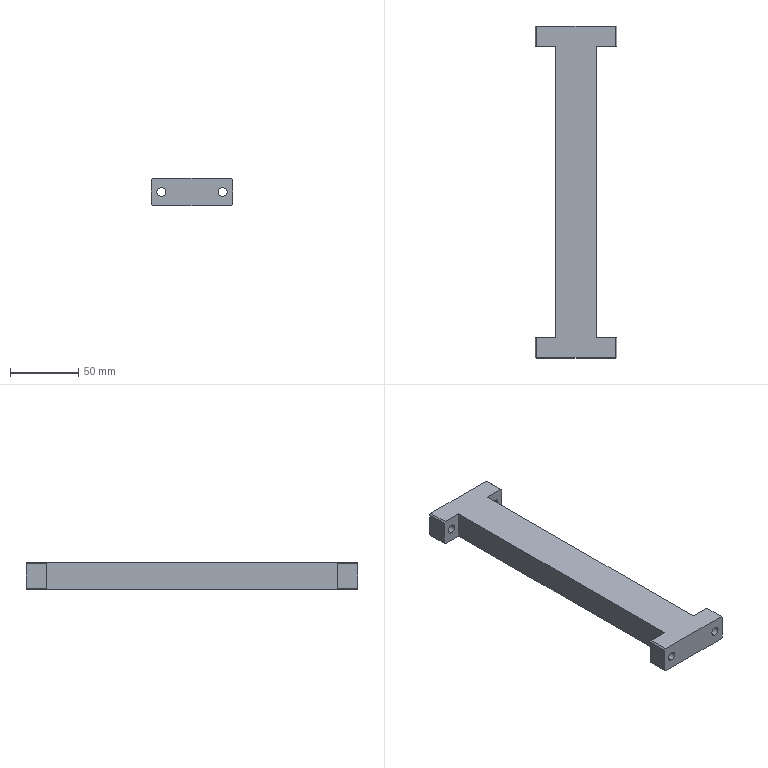Part | SolidWorks | features Chamfer 1, Extrusion 1, HoleWzd 1, ICE 1 | 1 solid | 30 faces | box 60 x 244 x 20 mm | volume 162287 mm3 | plane 22 | cylinder 8 | commonest cylinder face diameters 6.6 x8
STEP:
#1=CARTESIAN_POINT('',(-22.5,-122.,6.7));
#2=VERTEX_POINT('',#1);
#3=CARTESIAN_POINT('',(-22.5,-122.,13.3));
#4=VERTEX_POINT('',#3);
#5=CARTESIAN_POINT('',(-22.5,-122.,10.));
#6=DIRECTION('',(0.,1.,0.));
#7=DIRECTION('',(0.,0.,1.));
#8=AXIS2_PLACEMENT_3D('',#5,#6,#7);
#9=CIRCLE('',#8,3.3);
#10=EDGE_CURVE('',#2,#4,#9,.T.);
#11=ORIENTED_EDGE('',*,*,#10,.F.);
#12=CARTESIAN_POINT('',(-22.5,-107.,6.7));
#13=VERTEX_POINT('',#12);
#14=CARTESIAN_POINT('',(-22.5,122.,6.7));
#15=DIRECTION('',(0.,1.,0.));
#16=VECTOR('',#15,1000.);
#17=LINE('',#14,#16);
#18=EDGE_CURVE('',#2,#13,#17,.T.);
#19=ORIENTED_EDGE('',*,*,#18,.T.);
#20=CARTESIAN_POINT('',(-22.5,-107.,13.3));
#21=VERTEX_POINT('',#20);
#22=CARTESIAN_POINT('',(-22.5,-107.,10.));
#23=DIRECTION('',(0.,-1.,0.));
#24=DIRECTION('',(0.,0.,-1.));
#25=AXIS2_PLACEMENT_3D('',#22,#23,#24);
#26=CIRCLE('',#25,3.3);
#27=EDGE_CURVE('',#21,#13,#26,.T.);
#28=ORIENTED_EDGE('',*,*,#27,.F.);
#29=CARTESIAN_POINT('',(-22.5,122.,13.3));
#30=DIRECTION('',(0.,1.,0.));
#31=VECTOR('',#30,1000.);
#32=LINE('',#29,#31);
#33=EDGE_CURVE('',#4,#21,#32,.T.);
#34=ORIENTED_EDGE('',*,*,#33,.F.);
#35=EDGE_LOOP('',(#11,#19,#28,#34));
#36=FACE_OUTER_BOUND('',#35,.T.);
#37=CARTESIAN_POINT('',(-22.5,122.,10.));
#38=DIRECTION('',(0.,1.,0.));
#39=DIRECTION('',(0.,0.,1.));
#40=AXIS2_PLACEMENT_3D('',#37,#38,#39);
#41=CYLINDRICAL_SURFACE('',#40,3.3);
#42=ADVANCED_FACE('',(#36),#41,.F.);
#43=CARTESIAN_POINT('',(-22.5,107.,6.7));
#44=VERTEX_POINT('',#43);
#45=CARTESIAN_POINT('',(-22.5,107.,13.3));
#46=VERTEX_POINT('',#45);
#47=CARTESIAN_POINT('',(-22.5,107.,10.));
#48=DIRECTION('',(0.,1.,0.));
#49=DIRECTION('',(0.,0.,1.));
#50=AXIS2_PLACEMENT_3D('',#47,#48,#49);
#51=CIRCLE('',#50,3.3);
#52=EDGE_CURVE('',#44,#46,#51,.T.);
#53=ORIENTED_EDGE('',*,*,#52,.F.);
#54=CARTESIAN_POINT('',(-22.5,122.,6.7));
#55=VERTEX_POINT('',#54);
#56=CARTESIAN_POINT('',(-22.5,122.,6.7));
#57=DIRECTION('',(0.,1.,0.));
#58=VECTOR('',#57,1000.);
#59=LINE('',#56,#58);
#60=EDGE_CURVE('',#44,#55,#59,.T.);
#61=ORIENTED_EDGE('',*,*,#60,.T.);
#62=CARTESIAN_POINT('',(-22.5,122.,13.3));
#63=VERTEX_POINT('',#62);
#64=CARTESIAN_POINT('',(-22.5,122.,10.));
#65=DIRECTION('',(0.,1.,0.));
#66=DIRECTION('',(0.,0.,1.));
#67=AXIS2_PLACEMENT_3D('',#64,#65,#66);
#68=CIRCLE('',#67,3.3);
#69=EDGE_CURVE('',#55,#63,#68,.T.);
#70=ORIENTED_EDGE('',*,*,#69,.T.);
#71=CARTESIAN_POINT('',(-22.5,122.,13.3));
#72=DIRECTION('',(0.,1.,0.));
#73=VECTOR('',#72,1000.);
#74=LINE('',#71,#73);
#75=EDGE_CURVE('',#46,#63,#74,.T.);
#76=ORIENTED_EDGE('',*,*,#75,.F.);
#77=EDGE_LOOP('',(#53,#61,#70,#76));
#78=FACE_OUTER_BOUND('',#77,.T.);
#79=CARTESIAN_POINT('',(-22.5,122.,10.));
#80=DIRECTION('',(0.,1.,0.));
#81=DIRECTION('',(0.,0.,1.));
#82=AXIS2_PLACEMENT_3D('',#79,#80,#81);
#83=CYLINDRICAL_SURFACE('',#82,3.3);
#84=ADVANCED_FACE('',(#78),#83,.F.);
#85=CARTESIAN_POINT('',(22.5,107.,6.7));
#86=VERTEX_POINT('',#85);
#87=CARTESIAN_POINT('',(22.5,107.,13.3));
#88=VERTEX_POINT('',#87);
#89=CARTESIAN_POINT('',(22.5,107.,10.));
#90=DIRECTION('',(0.,1.,0.));
#91=DIRECTION('',(-1.,0.,0.));
#92=AXIS2_PLACEMENT_3D('',#89,#90,#91);
#93=CIRCLE('',#92,3.3);
#94=EDGE_CURVE('',#86,#88,#93,.T.);
#95=ORIENTED_EDGE('',*,*,#94,.F.);
#96=CARTESIAN_POINT('',(22.5,122.,6.7));
#97=VERTEX_POINT('',#96);
#98=CARTESIAN_POINT('',(22.5,122.,6.7));
#99=DIRECTION('',(0.,1.,0.));
#100=VECTOR('',#99,1000.);
#101=LINE('',#98,#100);
#102=EDGE_CURVE('',#86,#97,#101,.T.);
#103=ORIENTED_EDGE('',*,*,#102,.T.);
#104=CARTESIAN_POINT('',(22.5,122.,13.3));
#105=VERTEX_POINT('',#104);
#106=CARTESIAN_POINT('',(22.5,122.,10.));
#107=DIRECTION('',(0.,1.,0.));
#108=DIRECTION('',(0.,0.,1.));
#109=AXIS2_PLACEMENT_3D('',#106,#107,#108);
#110=CIRCLE('',#109,3.3);
#111=EDGE_CURVE('',#97,#105,#110,.T.);
#112=ORIENTED_EDGE('',*,*,#111,.T.);
#113=CARTESIAN_POINT('',(22.5,122.,13.3));
#114=DIRECTION('',(0.,1.,0.));
#115=VECTOR('',#114,1000.);
#116=LINE('',#113,#115);
#117=EDGE_CURVE('',#88,#105,#116,.T.);
#118=ORIENTED_EDGE('',*,*,#117,.F.);
#119=EDGE_LOOP('',(#95,#103,#112,#118));
#120=FACE_OUTER_BOUND('',#119,.T.);
#121=CARTESIAN_POINT('',(22.5,122.,10.));
#122=DIRECTION('',(0.,1.,0.));
#123=DIRECTION('',(0.,0.,1.));
#124=AXIS2_PLACEMENT_3D('',#121,#122,#123);
#125=CYLINDRICAL_SURFACE('',#124,3.3);
#126=ADVANCED_FACE('',(#120),#125,.F.);
#127=CARTESIAN_POINT('',(22.5,-122.,6.7));
#128=VERTEX_POINT('',#127);
#129=CARTESIAN_POINT('',(22.5,-122.,13.3));
#130=VERTEX_POINT('',#129);
#131=CARTESIAN_POINT('',(22.5,-122.,10.));
#132=DIRECTION('',(0.,1.,0.));
#133=DIRECTION('',(0.,0.,1.));
#134=AXIS2_PLACEMENT_3D('',#131,#132,#133);
#135=CIRCLE('',#134,3.3);
#136=EDGE_CURVE('',#128,#130,#135,.T.);
#137=ORIENTED_EDGE('',*,*,#136,.F.);
#138=CARTESIAN_POINT('',(22.5,-107.,6.7));
#139=VERTEX_POINT('',#138);
#140=CARTESIAN_POINT('',(22.5,122.,6.7));
#141=DIRECTION('',(0.,1.,0.));
#142=VECTOR('',#141,1000.);
#143=LINE('',#140,#142);
#144=EDGE_CURVE('',#128,#139,#143,.T.);
#145=ORIENTED_EDGE('',*,*,#144,.T.);
#146=CARTESIAN_POINT('',(22.5,-107.,13.3));
#147=VERTEX_POINT('',#146);
#148=CARTESIAN_POINT('',(22.5,-107.,10.));
#149=DIRECTION('',(0.,-1.,0.));
#150=DIRECTION('',(1.,0.,0.));
#151=AXIS2_PLACEMENT_3D('',#148,#149,#150);
#152=CIRCLE('',#151,3.3);
#153=EDGE_CURVE('',#147,#139,#152,.T.);
#154=ORIENTED_EDGE('',*,*,#153,.F.);
#155=CARTESIAN_POINT('',(22.5,122.,13.3));
#156=DIRECTION('',(0.,1.,0.));
#157=VECTOR('',#156,1000.);
#158=LINE('',#155,#157);
#159=EDGE_CURVE('',#130,#147,#158,.T.);
#160=ORIENTED_EDGE('',*,*,#159,.F.);
#161=EDGE_LOOP('',(#137,#145,#154,#160));
#162=FACE_OUTER_BOUND('',#161,.T.);
#163=CARTESIAN_POINT('',(22.5,122.,10.));
#164=DIRECTION('',(0.,1.,0.));
#165=DIRECTION('',(0.,0.,1.));
#166=AXIS2_PLACEMENT_3D('',#163,#164,#165);
#167=CYLINDRICAL_SURFACE('',#166,3.3);
#168=ADVANCED_FACE('',(#162),#167,.F.);
#169=CARTESIAN_POINT('',(30.,-122.,19.));
#170=VERTEX_POINT('',#169);
#171=CARTESIAN_POINT('',(30.,-122.,1.));
#172=VERTEX_POINT('',#171);
#173=CARTESIAN_POINT('',(30.,-122.,20.));
#174=DIRECTION('',(0.,0.,-1.));
#175=VECTOR('',#174,1000.);
#176=LINE('',#173,#175);
#177=EDGE_CURVE('',#170,#172,#176,.T.);
#178=ORIENTED_EDGE('',*,*,#177,.T.);
#179=CARTESIAN_POINT('',(30.,-107.,1.));
#180=VERTEX_POINT('',#179);
#181=CARTESIAN_POINT('',(30.,122.,1.));
#182=DIRECTION('',(0.,1.,0.));
#183=VECTOR('',#182,1000.);
#184=LINE('',#181,#183);
#185=EDGE_CURVE('',#172,#180,#184,.T.);
#186=ORIENTED_EDGE('',*,*,#185,.T.);
#187=CARTESIAN_POINT('',(30.,-107.,19.));
#188=VERTEX_POINT('',#187);
#189=CARTESIAN_POINT('',(30.,-107.,0.));
#190=DIRECTION('',(0.,0.,1.));
#191=VECTOR('',#190,1000.);
#192=LINE('',#189,#191);
#193=EDGE_CURVE('',#180,#188,#192,.T.);
#194=ORIENTED_EDGE('',*,*,#193,.T.);
#195=CARTESIAN_POINT('',(30.,-122.,19.));
#196=DIRECTION('',(0.,-1.,0.));
#197=VECTOR('',#196,1000.);
#198=LINE('',#195,#197);
#199=EDGE_CURVE('',#188,#170,#198,.T.);
#200=ORIENTED_EDGE('',*,*,#199,.T.);
#201=EDGE_LOOP('',(#178,#186,#194,#200));
#202=FACE_OUTER_BOUND('',#201,.T.);
#203=CARTESIAN_POINT('',(30.,122.,20.));
#204=DIRECTION('',(-1.,0.,0.));
#205=DIRECTION('',(0.,-1.,0.));
#206=AXIS2_PLACEMENT_3D('',#203,#204,#205);
#207=PLANE('',#206);
#208=ADVANCED_FACE('',(#202),#207,.F.);
#209=CARTESIAN_POINT('',(-30.,122.,19.));
#210=VERTEX_POINT('',#209);
#211=CARTESIAN_POINT('',(-30.,122.,1.));
#212=VERTEX_POINT('',#211);
#213=CARTESIAN_POINT('',(-30.,122.,20.));
#214=DIRECTION('',(0.,0.,-1.));
#215=VECTOR('',#214,1000.);
#216=LINE('',#213,#215);
#217=EDGE_CURVE('',#210,#212,#216,.T.);
#218=ORIENTED_EDGE('',*,*,#217,.T.);
#219=CARTESIAN_POINT('',(-30.,107.,1.));
#220=VERTEX_POINT('',#219);
#221=CARTESIAN_POINT('',(-30.,122.,1.));
#222=DIRECTION('',(0.,-1.,0.));
#223=VECTOR('',#222,1000.);
#224=LINE('',#221,#223);
#225=EDGE_CURVE('',#212,#220,#224,.T.);
#226=ORIENTED_EDGE('',*,*,#225,.T.);
#227=CARTESIAN_POINT('',(-30.,107.,19.));
#228=VERTEX_POINT('',#227);
#229=CARTESIAN_POINT('',(-30.,107.,0.));
#230=DIRECTION('',(0.,0.,1.));
#231=VECTOR('',#230,1000.);
#232=LINE('',#229,#231);
#233=EDGE_CURVE('',#220,#228,#232,.T.);
#234=ORIENTED_EDGE('',*,*,#233,.T.);
#235=CARTESIAN_POINT('',(-30.,122.,19.));
#236=DIRECTION('',(0.,1.,0.));
#237=VECTOR('',#236,1000.);
#238=LINE('',#235,#237);
#239=EDGE_CURVE('',#228,#210,#238,.T.);
#240=ORIENTED_EDGE('',*,*,#239,.T.);
#241=EDGE_LOOP('',(#218,#226,#234,#240));
#242=FACE_OUTER_BOUND('',#241,.T.);
#243=CARTESIAN_POINT('',(-30.,122.,20.));
#244=DIRECTION('',(1.,0.,0.));
#245=DIRECTION('',(0.,1.,0.));
#246=AXIS2_PLACEMENT_3D('',#243,#244,#245);
#247=PLANE('',#246);
#248=ADVANCED_FACE('',(#242),#247,.F.);
#249=CARTESIAN_POINT('',(30.,122.,19.));
#250=VERTEX_POINT('',#249);
#251=CARTESIAN_POINT('',(30.,122.,1.));
#252=VERTEX_POINT('',#251);
#253=CARTESIAN_POINT('',(30.,122.,20.));
#254=DIRECTION('',(0.,0.,-1.));
#255=VECTOR('',#254,1000.);
#256=LINE('',#253,#255);
#257=EDGE_CURVE('',#250,#252,#256,.T.);
#258=ORIENTED_EDGE('',*,*,#257,.F.);
#259=CARTESIAN_POINT('',(30.,107.,19.));
#260=VERTEX_POINT('',#259);
#261=CARTESIAN_POINT('',(30.,107.,19.));
#262=DIRECTION('',(0.,-1.,0.));
#263=VECTOR('',#262,1000.);
#264=LINE('',#261,#263);
#265=EDGE_CURVE('',#250,#260,#264,.T.);
#266=ORIENTED_EDGE('',*,*,#265,.T.);
#267=CARTESIAN_POINT('',(30.,107.,1.));
#268=VERTEX_POINT('',#267);
#269=CARTESIAN_POINT('',(30.,107.,0.));
#270=DIRECTION('',(0.,0.,1.));
#271=VECTOR('',#270,1000.);
#272=LINE('',#269,#271);
#273=EDGE_CURVE('',#268,#260,#272,.T.);
#274=ORIENTED_EDGE('',*,*,#273,.F.);
#275=CARTESIAN_POINT('',(30.,122.,1.));
#276=DIRECTION('',(0.,1.,0.));
#277=VECTOR('',#276,1000.);
#278=LINE('',#275,#277);
#279=EDGE_CURVE('',#268,#252,#278,.T.);
#280=ORIENTED_EDGE('',*,*,#279,.T.);
#281=EDGE_LOOP('',(#258,#266,#274,#280));
#282=FACE_OUTER_BOUND('',#281,.T.);
#283=CARTESIAN_POINT('',(30.,122.,20.));
#284=DIRECTION('',(-1.,0.,0.));
#285=DIRECTION('',(0.,-1.,0.));
#286=AXIS2_PLACEMENT_3D('',#283,#284,#285);
#287=PLANE('',#286);
#288=ADVANCED_FACE('',(#282),#287,.F.);
#289=CARTESIAN_POINT('',(-22.5,122.,10.));
#290=DIRECTION('',(0.,1.,0.));
#291=DIRECTION('',(0.,0.,1.));
#292=AXIS2_PLACEMENT_3D('',#289,#290,#291);
#293=CIRCLE('',#292,3.3);
#294=EDGE_CURVE('',#63,#55,#293,.T.);
#295=ORIENTED_EDGE('',*,*,#294,.F.);
#296=ORIENTED_EDGE('',*,*,#69,.F.);
#297=EDGE_LOOP('',(#295,#296));
#298=FACE_BOUND('',#297,.T.);
#299=CARTESIAN_POINT('',(22.5,122.,10.));
#300=DIRECTION('',(0.,1.,0.));
#301=DIRECTION('',(0.,0.,1.));
#302=AXIS2_PLACEMENT_3D('',#299,#300,#301);
#303=CIRCLE('',#302,3.3);
#304=EDGE_CURVE('',#105,#97,#303,.T.);
#305=ORIENTED_EDGE('',*,*,#304,.F.);
#306=ORIENTED_EDGE('',*,*,#111,.F.);
#307=EDGE_LOOP('',(#305,#306));
#308=FACE_BOUND('',#307,.T.);
#309=CARTESIAN_POINT('',(29.,122.,20.));
#310=VERTEX_POINT('',#309);
#311=CARTESIAN_POINT('',(-29.,122.,20.));
#312=VERTEX_POINT('',#311);
#313=CARTESIAN_POINT('',(-30.,122.,20.));
#314=DIRECTION('',(-1.,0.,0.));
#315=VECTOR('',#314,1000.);
#316=LINE('',#313,#315);
#317=EDGE_CURVE('',#310,#312,#316,.T.);
#318=ORIENTED_EDGE('',*,*,#317,.F.);
#319=CARTESIAN_POINT('',(29.,122.,20.));
#320=DIRECTION('',(0.7071,0.,-0.7071));
#321=VECTOR('',#320,1000.);
#322=LINE('',#319,#321);
#323=EDGE_CURVE('',#310,#250,#322,.T.);
#324=ORIENTED_EDGE('',*,*,#323,.T.);
#325=ORIENTED_EDGE('',*,*,#257,.T.);
#326=CARTESIAN_POINT('',(29.,122.,0.));
#327=VERTEX_POINT('',#326);
#328=CARTESIAN_POINT('',(30.,122.,1.));
#329=DIRECTION('',(-0.7071,0.,-0.7071));
#330=VECTOR('',#329,1000.);
#331=LINE('',#328,#330);
#332=EDGE_CURVE('',#252,#327,#331,.T.);
#333=ORIENTED_EDGE('',*,*,#332,.T.);
#334=CARTESIAN_POINT('',(-29.,122.,0.));
#335=VERTEX_POINT('',#334);
#336=CARTESIAN_POINT('',(-30.,122.,0.));
#337=DIRECTION('',(-1.,0.,0.));
#338=VECTOR('',#337,1000.);
#339=LINE('',#336,#338);
#340=EDGE_CURVE('',#327,#335,#339,.T.);
#341=ORIENTED_EDGE('',*,*,#340,.T.);
#342=CARTESIAN_POINT('',(-30.,122.,1.));
#343=DIRECTION('',(-0.7071,0.,0.7071));
#344=VECTOR('',#343,1000.);
#345=LINE('',#342,#344);
#346=EDGE_CURVE('',#335,#212,#345,.T.);
#347=ORIENTED_EDGE('',*,*,#346,.T.);
#348=ORIENTED_EDGE('',*,*,#217,.F.);
#349=CARTESIAN_POINT('',(-29.,122.,20.));
#350=DIRECTION('',(0.7071,0.,0.7071));
#351=VECTOR('',#350,1000.);
#352=LINE('',#349,#351);
#353=EDGE_CURVE('',#210,#312,#352,.T.);
#354=ORIENTED_EDGE('',*,*,#353,.T.);
#355=EDGE_LOOP('',(#318,#324,#325,#333,#341,#347,#348,#354));
#356=FACE_OUTER_BOUND('',#355,.T.);
#357=CARTESIAN_POINT('',(-30.,122.,20.));
#358=DIRECTION('',(0.,-1.,0.));
#359=DIRECTION('',(0.,0.,-1.));
#360=AXIS2_PLACEMENT_3D('',#357,#358,#359);
#361=PLANE('',#360);
#362=ADVANCED_FACE('',(#298,#308,#356),#361,.F.);
#363=CARTESIAN_POINT('',(-30.,-122.,19.));
#364=VERTEX_POINT('',#363);
#365=CARTESIAN_POINT('',(-30.,-122.,1.));
#366=VERTEX_POINT('',#365);
#367=CARTESIAN_POINT('',(-30.,-122.,20.));
#368=DIRECTION('',(0.,0.,-1.));
#369=VECTOR('',#368,1000.);
#370=LINE('',#367,#369);
#371=EDGE_CURVE('',#364,#366,#370,.T.);
#372=ORIENTED_EDGE('',*,*,#371,.F.);
#373=CARTESIAN_POINT('',(-30.,-107.,19.));
#374=VERTEX_POINT('',#373);
#375=CARTESIAN_POINT('',(-30.,-107.,19.));
#376=DIRECTION('',(0.,1.,0.));
#377=VECTOR('',#376,1000.);
#378=LINE('',#375,#377);
#379=EDGE_CURVE('',#364,#374,#378,.T.);
#380=ORIENTED_EDGE('',*,*,#379,.T.);
#381=CARTESIAN_POINT('',(-30.,-107.,1.));
#382=VERTEX_POINT('',#381);
#383=CARTESIAN_POINT('',(-30.,-107.,0.));
#384=DIRECTION('',(0.,0.,1.));
#385=VECTOR('',#384,1000.);
#386=LINE('',#383,#385);
#387=EDGE_CURVE('',#382,#374,#386,.T.);
#388=ORIENTED_EDGE('',*,*,#387,.F.);
#389=CARTESIAN_POINT('',(-30.,122.,1.));
#390=DIRECTION('',(0.,-1.,0.));
#391=VECTOR('',#390,1000.);
#392=LINE('',#389,#391);
#393=EDGE_CURVE('',#382,#366,#392,.T.);
#394=ORIENTED_EDGE('',*,*,#393,.T.);
#395=EDGE_LOOP('',(#372,#380,#388,#394));
#396=FACE_OUTER_BOUND('',#395,.T.);
#397=CARTESIAN_POINT('',(-30.,122.,20.));
#398=DIRECTION('',(1.,0.,0.));
#399=DIRECTION('',(0.,1.,0.));
#400=AXIS2_PLACEMENT_3D('',#397,#398,#399);
#401=PLANE('',#400);
#402=ADVANCED_FACE('',(#396),#401,.F.);
#403=CARTESIAN_POINT('',(-22.5,-122.,10.));
#404=DIRECTION('',(0.,1.,0.));
#405=DIRECTION('',(0.,0.,1.));
#406=AXIS2_PLACEMENT_3D('',#403,#404,#405);
#407=CIRCLE('',#406,3.3);
#408=EDGE_CURVE('',#4,#2,#407,.T.);
#409=ORIENTED_EDGE('',*,*,#408,.T.);
#410=ORIENTED_EDGE('',*,*,#10,.T.);
#411=EDGE_LOOP('',(#409,#410));
#412=FACE_BOUND('',#411,.T.);
#413=CARTESIAN_POINT('',(22.5,-122.,10.));
#414=DIRECTION('',(0.,1.,0.));
#415=DIRECTION('',(0.,0.,1.));
#416=AXIS2_PLACEMENT_3D('',#413,#414,#415);
#417=CIRCLE('',#416,3.3);
#418=EDGE_CURVE('',#130,#128,#417,.T.);
#419=ORIENTED_EDGE('',*,*,#418,.T.);
#420=ORIENTED_EDGE('',*,*,#136,.T.);
#421=EDGE_LOOP('',(#419,#420));
#422=FACE_BOUND('',#421,.T.);
#423=CARTESIAN_POINT('',(-29.,-122.,20.));
#424=VERTEX_POINT('',#423);
#425=CARTESIAN_POINT('',(29.,-122.,20.));
#426=VERTEX_POINT('',#425);
#427=CARTESIAN_POINT('',(-30.,-122.,20.));
#428=DIRECTION('',(1.,0.,0.));
#429=VECTOR('',#428,1000.);
#430=LINE('',#427,#429);
#431=EDGE_CURVE('',#424,#426,#430,.T.);
#432=ORIENTED_EDGE('',*,*,#431,.F.);
#433=CARTESIAN_POINT('',(-29.,-122.,20.));
#434=DIRECTION('',(-0.7071,0.,-0.7071));
#435=VECTOR('',#434,1000.);
#436=LINE('',#433,#435);
#437=EDGE_CURVE('',#424,#364,#436,.T.);
#438=ORIENTED_EDGE('',*,*,#437,.T.);
#439=ORIENTED_EDGE('',*,*,#371,.T.);
#440=CARTESIAN_POINT('',(-29.,-122.,0.));
#441=VERTEX_POINT('',#440);
#442=CARTESIAN_POINT('',(-30.,-122.,1.));
#443=DIRECTION('',(0.7071,0.,-0.7071));
#444=VECTOR('',#443,1000.);
#445=LINE('',#442,#444);
#446=EDGE_CURVE('',#366,#441,#445,.T.);
#447=ORIENTED_EDGE('',*,*,#446,.T.);
#448=CARTESIAN_POINT('',(29.,-122.,0.));
#449=VERTEX_POINT('',#448);
#450=CARTESIAN_POINT('',(-30.,-122.,0.));
#451=DIRECTION('',(1.,0.,0.));
#452=VECTOR('',#451,1000.);
#453=LINE('',#450,#452);
#454=EDGE_CURVE('',#441,#449,#453,.T.);
#455=ORIENTED_EDGE('',*,*,#454,.T.);
#456=CARTESIAN_POINT('',(30.,-122.,1.));
#457=DIRECTION('',(0.7071,0.,0.7071));
#458=VECTOR('',#457,1000.);
#459=LINE('',#456,#458);
#460=EDGE_CURVE('',#449,#172,#459,.T.);
#461=ORIENTED_EDGE('',*,*,#460,.T.);
#462=ORIENTED_EDGE('',*,*,#177,.F.);
#463=CARTESIAN_POINT('',(29.,-122.,20.));
#464=DIRECTION('',(-0.7071,0.,0.7071));
#465=VECTOR('',#464,1000.);
#466=LINE('',#463,#465);
#467=EDGE_CURVE('',#170,#426,#466,.T.);
#468=ORIENTED_EDGE('',*,*,#467,.T.);
#469=EDGE_LOOP('',(#432,#438,#439,#447,#455,#461,#462,#468));
#470=FACE_OUTER_BOUND('',#469,.T.);
#471=CARTESIAN_POINT('',(-30.,-122.,20.));
#472=DIRECTION('',(0.,1.,0.));
#473=DIRECTION('',(0.,0.,1.));
#474=AXIS2_PLACEMENT_3D('',#471,#472,#473);
#475=PLANE('',#474);
#476=ADVANCED_FACE('',(#412,#422,#470),#475,.F.);
#477=CARTESIAN_POINT('',(-29.,-107.,20.));
#478=VERTEX_POINT('',#477);
#479=CARTESIAN_POINT('',(-15.,-107.,20.));
#480=VERTEX_POINT('',#479);
#481=CARTESIAN_POINT('',(-30.,-107.,20.));
#482=DIRECTION('',(1.,0.,0.));
#483=VECTOR('',#482,1000.);
#484=LINE('',#481,#483);
#485=EDGE_CURVE('',#478,#480,#484,.T.);
#486=ORIENTED_EDGE('',*,*,#485,.F.);
#487=CARTESIAN_POINT('',(-29.,-122.,20.));
#488=DIRECTION('',(0.,-1.,0.));
#489=VECTOR('',#488,1000.);
#490=LINE('',#487,#489);
#491=EDGE_CURVE('',#478,#424,#490,.T.);
#492=ORIENTED_EDGE('',*,*,#491,.T.);
#493=ORIENTED_EDGE('',*,*,#431,.T.);
#494=CARTESIAN_POINT('',(29.,-107.,20.));
#495=VERTEX_POINT('',#494);
#496=CARTESIAN_POINT('',(29.,-107.,20.));
#497=DIRECTION('',(0.,1.,0.));
#498=VECTOR('',#497,1000.);
#499=LINE('',#496,#498);
#500=EDGE_CURVE('',#426,#495,#499,.T.);
#501=ORIENTED_EDGE('',*,*,#500,.T.);
#502=CARTESIAN_POINT('',(15.,-107.,20.));
#503=VERTEX_POINT('',#502);
#504=CARTESIAN_POINT('',(30.,-107.,20.));
#505=DIRECTION('',(1.,0.,0.));
#506=VECTOR('',#505,1000.);
#507=LINE('',#504,#506);
#508=EDGE_CURVE('',#503,#495,#507,.T.);
#509=ORIENTED_EDGE('',*,*,#508,.F.);
#510=CARTESIAN_POINT('',(15.,107.,20.));
#511=VERTEX_POINT('',#510);
#512=CARTESIAN_POINT('',(15.,107.,20.));
#513=DIRECTION('',(0.,-1.,0.));
#514=VECTOR('',#513,1000.);
#515=LINE('',#512,#514);
#516=EDGE_CURVE('',#511,#503,#515,.T.);
#517=ORIENTED_EDGE('',*,*,#516,.F.);
#518=CARTESIAN_POINT('',(29.,107.,20.));
#519=VERTEX_POINT('',#518);
#520=CARTESIAN_POINT('',(30.,107.,20.));
#521=DIRECTION('',(-1.,0.,0.));
#522=VECTOR('',#521,1000.);
#523=LINE('',#520,#522);
#524=EDGE_CURVE('',#519,#511,#523,.T.);
#525=ORIENTED_EDGE('',*,*,#524,.F.);
#526=CARTESIAN_POINT('',(29.,122.,20.));
#527=DIRECTION('',(0.,1.,0.));
#528=VECTOR('',#527,1000.);
#529=LINE('',#526,#528);
#530=EDGE_CURVE('',#519,#310,#529,.T.);
#531=ORIENTED_EDGE('',*,*,#530,.T.);
#532=ORIENTED_EDGE('',*,*,#317,.T.);
#533=CARTESIAN_POINT('',(-29.,107.,20.));
#534=VERTEX_POINT('',#533);
#535=CARTESIAN_POINT('',(-29.,107.,20.));
#536=DIRECTION('',(0.,-1.,0.));
#537=VECTOR('',#536,1000.);
#538=LINE('',#535,#537);
#539=EDGE_CURVE('',#312,#534,#538,.T.);
#540=ORIENTED_EDGE('',*,*,#539,.T.);
#541=CARTESIAN_POINT('',(-15.,107.,20.));
#542=VERTEX_POINT('',#541);
#543=CARTESIAN_POINT('',(-30.,107.,20.));
#544=DIRECTION('',(-1.,0.,0.));
#545=VECTOR('',#544,1000.);
#546=LINE('',#543,#545);
#547=EDGE_CURVE('',#542,#534,#546,.T.);
#548=ORIENTED_EDGE('',*,*,#547,.F.);
#549=CARTESIAN_POINT('',(-15.,107.,20.));
#550=DIRECTION('',(0.,1.,0.));
#551=VECTOR('',#550,1000.);
#552=LINE('',#549,#551);
#553=EDGE_CURVE('',#480,#542,#552,.T.);
#554=ORIENTED_EDGE('',*,*,#553,.F.);
#555=EDGE_LOOP('',(#486,#492,#493,#501,#509,#517,#525,#531,#532,#540,#548,#554));
#556=FACE_OUTER_BOUND('',#555,.T.);
#557=CARTESIAN_POINT('',(0.,0.,20.));
#558=DIRECTION('',(0.,0.,1.));
#559=DIRECTION('',(1.,0.,0.));
#560=AXIS2_PLACEMENT_3D('',#557,#558,#559);
#561=PLANE('',#560);
#562=ADVANCED_FACE('',(#556),#561,.T.);
#563=ORIENTED_EDGE('',*,*,#454,.F.);
#564=CARTESIAN_POINT('',(-29.,-107.,0.));
#565=VERTEX_POINT('',#564);
#566=CARTESIAN_POINT('',(-29.,0.,0.));
#567=DIRECTION('',(0.,1.,0.));
#568=VECTOR('',#567,1000.);
#569=LINE('',#566,#568);
#570=EDGE_CURVE('',#441,#565,#569,.T.);
#571=ORIENTED_EDGE('',*,*,#570,.T.);
#572=CARTESIAN_POINT('',(-15.,-107.,0.));
#573=VERTEX_POINT('',#572);
#574=CARTESIAN_POINT('',(-30.,-107.,0.));
#575=DIRECTION('',(1.,0.,0.));
#576=VECTOR('',#575,1000.);
#577=LINE('',#574,#576);
#578=EDGE_CURVE('',#565,#573,#577,.T.);
#579=ORIENTED_EDGE('',*,*,#578,.T.);
#580=CARTESIAN_POINT('',(-15.,107.,0.));
#581=VERTEX_POINT('',#580);
#582=CARTESIAN_POINT('',(-15.,107.,0.));
#583=DIRECTION('',(0.,1.,0.));
#584=VECTOR('',#583,1000.);
#585=LINE('',#582,#584);
#586=EDGE_CURVE('',#573,#581,#585,.T.);
#587=ORIENTED_EDGE('',*,*,#586,.T.);
#588=CARTESIAN_POINT('',(-29.,107.,0.));
#589=VERTEX_POINT('',#588);
#590=CARTESIAN_POINT('',(-30.,107.,0.));
#591=DIRECTION('',(-1.,0.,0.));
#592=VECTOR('',#591,1000.);
#593=LINE('',#590,#592);
#594=EDGE_CURVE('',#581,#589,#593,.T.);
#595=ORIENTED_EDGE('',*,*,#594,.T.);
#596=CARTESIAN_POINT('',(-29.,0.,0.));
#597=DIRECTION('',(0.,1.,0.));
#598=VECTOR('',#597,1000.);
#599=LINE('',#596,#598);
#600=EDGE_CURVE('',#589,#335,#599,.T.);
#601=ORIENTED_EDGE('',*,*,#600,.T.);
#602=ORIENTED_EDGE('',*,*,#340,.F.);
#603=CARTESIAN_POINT('',(29.,107.,0.));
#604=VERTEX_POINT('',#603);
#605=CARTESIAN_POINT('',(29.,0.,0.));
#606=DIRECTION('',(0.,-1.,0.));
#607=VECTOR('',#606,1000.);
#608=LINE('',#605,#607);
#609=EDGE_CURVE('',#327,#604,#608,.T.);
#610=ORIENTED_EDGE('',*,*,#609,.T.);
#611=CARTESIAN_POINT('',(15.,107.,0.));
#612=VERTEX_POINT('',#611);
#613=CARTESIAN_POINT('',(30.,107.,0.));
#614=DIRECTION('',(-1.,0.,0.));
#615=VECTOR('',#614,1000.);
#616=LINE('',#613,#615);
#617=EDGE_CURVE('',#604,#612,#616,.T.);
#618=ORIENTED_EDGE('',*,*,#617,.T.);
#619=CARTESIAN_POINT('',(15.,-107.,0.));
#620=VERTEX_POINT('',#619);
#621=CARTESIAN_POINT('',(15.,107.,0.));
#622=DIRECTION('',(0.,-1.,0.));
#623=VECTOR('',#622,1000.);
#624=LINE('',#621,#623);
#625=EDGE_CURVE('',#612,#620,#624,.T.);
#626=ORIENTED_EDGE('',*,*,#625,.T.);
#627=CARTESIAN_POINT('',(29.,-107.,0.));
#628=VERTEX_POINT('',#627);
#629=CARTESIAN_POINT('',(30.,-107.,0.));
#630=DIRECTION('',(1.,0.,0.));
#631=VECTOR('',#630,1000.);
#632=LINE('',#629,#631);
#633=EDGE_CURVE('',#620,#628,#632,.T.);
#634=ORIENTED_EDGE('',*,*,#633,.T.);
#635=CARTESIAN_POINT('',(29.,0.,0.));
#636=DIRECTION('',(0.,-1.,0.));
#637=VECTOR('',#636,1000.);
#638=LINE('',#635,#637);
#639=EDGE_CURVE('',#628,#449,#638,.T.);
#640=ORIENTED_EDGE('',*,*,#639,.T.);
#641=EDGE_LOOP('',(#563,#571,#579,#587,#595,#601,#602,#610,#618,#626,#634,#640));
#642=FACE_OUTER_BOUND('',#641,.T.);
#643=CARTESIAN_POINT('',(0.,0.,0.));
#644=DIRECTION('',(0.,0.,1.));
#645=DIRECTION('',(1.,0.,0.));
#646=AXIS2_PLACEMENT_3D('',#643,#644,#645);
#647=PLANE('',#646);
#648=ADVANCED_FACE('',(#642),#647,.F.);
#649=ORIENTED_EDGE('',*,*,#153,.T.);
#650=CARTESIAN_POINT('',(22.5,-107.,10.));
#651=DIRECTION('',(0.,-1.,0.));
#652=DIRECTION('',(1.,0.,0.));
#653=AXIS2_PLACEMENT_3D('',#650,#651,#652);
#654=CIRCLE('',#653,3.3);
#655=EDGE_CURVE('',#139,#147,#654,.T.);
#656=ORIENTED_EDGE('',*,*,#655,.T.);
#657=EDGE_LOOP('',(#649,#656));
#658=FACE_BOUND('',#657,.T.);
#659=ORIENTED_EDGE('',*,*,#193,.F.);
#660=CARTESIAN_POINT('',(30.,-107.,1.));
#661=DIRECTION('',(-0.7071,0.,-0.7071));
#662=VECTOR('',#661,1000.);
#663=LINE('',#660,#662);
#664=EDGE_CURVE('',#180,#628,#663,.T.);
#665=ORIENTED_EDGE('',*,*,#664,.T.);
#666=ORIENTED_EDGE('',*,*,#633,.F.);
#667=CARTESIAN_POINT('',(15.,-107.,0.));
#668=DIRECTION('',(0.,0.,1.));
#669=VECTOR('',#668,1000.);
#670=LINE('',#667,#669);
#671=EDGE_CURVE('',#620,#503,#670,.T.);
#672=ORIENTED_EDGE('',*,*,#671,.T.);
#673=ORIENTED_EDGE('',*,*,#508,.T.);
#674=CARTESIAN_POINT('',(29.,-107.,20.));
#675=DIRECTION('',(0.7071,0.,-0.7071));
#676=VECTOR('',#675,1000.);
#677=LINE('',#674,#676);
#678=EDGE_CURVE('',#495,#188,#677,.T.);
#679=ORIENTED_EDGE('',*,*,#678,.T.);
#680=EDGE_LOOP('',(#659,#665,#666,#672,#673,#679));
#681=FACE_OUTER_BOUND('',#680,.T.);
#682=CARTESIAN_POINT('',(30.,-107.,0.));
#683=DIRECTION('',(0.,-1.,0.));
#684=DIRECTION('',(1.,0.,0.));
#685=AXIS2_PLACEMENT_3D('',#682,#683,#684);
#686=PLANE('',#685);
#687=ADVANCED_FACE('',(#658,#681),#686,.F.);
#688=ORIENTED_EDGE('',*,*,#516,.T.);
#689=ORIENTED_EDGE('',*,*,#671,.F.);
#690=ORIENTED_EDGE('',*,*,#625,.F.);
#691=CARTESIAN_POINT('',(15.,107.,0.));
#692=DIRECTION('',(0.,0.,1.));
#693=VECTOR('',#692,1000.);
#694=LINE('',#691,#693);
#695=EDGE_CURVE('',#612,#511,#694,.T.);
#696=ORIENTED_EDGE('',*,*,#695,.T.);
#697=EDGE_LOOP('',(#688,#689,#690,#696));
#698=FACE_OUTER_BOUND('',#697,.T.);
#699=CARTESIAN_POINT('',(15.,107.,0.));
#700=DIRECTION('',(-1.,0.,0.));
#701=DIRECTION('',(0.,0.,1.));
#702=AXIS2_PLACEMENT_3D('',#699,#700,#701);
#703=PLANE('',#702);
#704=ADVANCED_FACE('',(#698),#703,.F.);
#705=CARTESIAN_POINT('',(22.5,107.,10.));
#706=DIRECTION('',(0.,1.,0.));
#707=DIRECTION('',(-1.,0.,0.));
#708=AXIS2_PLACEMENT_3D('',#705,#706,#707);
#709=CIRCLE('',#708,3.3);
#710=EDGE_CURVE('',#88,#86,#709,.T.);
#711=ORIENTED_EDGE('',*,*,#710,.T.);
#712=ORIENTED_EDGE('',*,*,#94,.T.);
#713=EDGE_LOOP('',(#711,#712));
#714=FACE_BOUND('',#713,.T.);
#715=ORIENTED_EDGE('',*,*,#273,.T.);
#716=CARTESIAN_POINT('',(29.,107.,20.));
#717=DIRECTION('',(-0.7071,0.,0.7071));
#718=VECTOR('',#717,1000.);
#719=LINE('',#716,#718);
#720=EDGE_CURVE('',#260,#519,#719,.T.);
#721=ORIENTED_EDGE('',*,*,#720,.T.);
#722=ORIENTED_EDGE('',*,*,#524,.T.);
#723=ORIENTED_EDGE('',*,*,#695,.F.);
#724=ORIENTED_EDGE('',*,*,#617,.F.);
#725=CARTESIAN_POINT('',(30.,107.,1.));
#726=DIRECTION('',(0.7071,0.,0.7071));
#727=VECTOR('',#726,1000.);
#728=LINE('',#725,#727);
#729=EDGE_CURVE('',#604,#268,#728,.T.);
#730=ORIENTED_EDGE('',*,*,#729,.T.);
#731=EDGE_LOOP('',(#715,#721,#722,#723,#724,#730));
#732=FACE_OUTER_BOUND('',#731,.T.);
#733=CARTESIAN_POINT('',(30.,107.,0.));
#734=DIRECTION('',(0.,1.,0.));
#735=DIRECTION('',(-1.,0.,0.));
#736=AXIS2_PLACEMENT_3D('',#733,#734,#735);
#737=PLANE('',#736);
#738=ADVANCED_FACE('',(#714,#732),#737,.F.);
#739=CARTESIAN_POINT('',(-22.5,107.,10.));
#740=DIRECTION('',(0.,1.,0.));
#741=DIRECTION('',(0.,0.,1.));
#742=AXIS2_PLACEMENT_3D('',#739,#740,#741);
#743=CIRCLE('',#742,3.3);
#744=EDGE_CURVE('',#46,#44,#743,.T.);
#745=ORIENTED_EDGE('',*,*,#744,.T.);
#746=ORIENTED_EDGE('',*,*,#52,.T.);
#747=EDGE_LOOP('',(#745,#746));
#748=FACE_BOUND('',#747,.T.);
#749=ORIENTED_EDGE('',*,*,#233,.F.);
#750=CARTESIAN_POINT('',(-30.,107.,1.));
#751=DIRECTION('',(0.7071,0.,-0.7071));
#752=VECTOR('',#751,1000.);
#753=LINE('',#750,#752);
#754=EDGE_CURVE('',#220,#589,#753,.T.);
#755=ORIENTED_EDGE('',*,*,#754,.T.);
#756=ORIENTED_EDGE('',*,*,#594,.F.);
#757=CARTESIAN_POINT('',(-15.,107.,0.));
#758=DIRECTION('',(0.,0.,1.));
#759=VECTOR('',#758,1000.);
#760=LINE('',#757,#759);
#761=EDGE_CURVE('',#581,#542,#760,.T.);
#762=ORIENTED_EDGE('',*,*,#761,.T.);
#763=ORIENTED_EDGE('',*,*,#547,.T.);
#764=CARTESIAN_POINT('',(-29.,107.,20.));
#765=DIRECTION('',(-0.7071,0.,-0.7071));
#766=VECTOR('',#765,1000.);
#767=LINE('',#764,#766);
#768=EDGE_CURVE('',#534,#228,#767,.T.);
#769=ORIENTED_EDGE('',*,*,#768,.T.);
#770=EDGE_LOOP('',(#749,#755,#756,#762,#763,#769));
#771=FACE_OUTER_BOUND('',#770,.T.);
#772=CARTESIAN_POINT('',(-30.,107.,0.));
#773=DIRECTION('',(0.,1.,0.));
#774=DIRECTION('',(0.,0.,1.));
#775=AXIS2_PLACEMENT_3D('',#772,#773,#774);
#776=PLANE('',#775);
#777=ADVANCED_FACE('',(#748,#771),#776,.F.);
#778=ORIENTED_EDGE('',*,*,#553,.T.);
#779=ORIENTED_EDGE('',*,*,#761,.F.);
#780=ORIENTED_EDGE('',*,*,#586,.F.);
#781=CARTESIAN_POINT('',(-15.,-107.,0.));
#782=DIRECTION('',(0.,0.,1.));
#783=VECTOR('',#782,1000.);
#784=LINE('',#781,#783);
#785=EDGE_CURVE('',#573,#480,#784,.T.);
#786=ORIENTED_EDGE('',*,*,#785,.T.);
#787=EDGE_LOOP('',(#778,#779,#780,#786));
#788=FACE_OUTER_BOUND('',#787,.T.);
#789=CARTESIAN_POINT('',(-15.,107.,0.));
#790=DIRECTION('',(1.,0.,0.));
#791=DIRECTION('',(0.,0.,-1.));
#792=AXIS2_PLACEMENT_3D('',#789,#790,#791);
#793=PLANE('',#792);
#794=ADVANCED_FACE('',(#788),#793,.F.);
#795=ORIENTED_EDGE('',*,*,#27,.T.);
#796=CARTESIAN_POINT('',(-22.5,-107.,10.));
#797=DIRECTION('',(0.,-1.,0.));
#798=DIRECTION('',(0.,0.,-1.));
#799=AXIS2_PLACEMENT_3D('',#796,#797,#798);
#800=CIRCLE('',#799,3.3);
#801=EDGE_CURVE('',#13,#21,#800,.T.);
#802=ORIENTED_EDGE('',*,*,#801,.T.);
#803=EDGE_LOOP('',(#795,#802));
#804=FACE_BOUND('',#803,.T.);
#805=ORIENTED_EDGE('',*,*,#387,.T.);
#806=CARTESIAN_POINT('',(-29.,-107.,20.));
#807=DIRECTION('',(0.7071,0.,0.7071));
#808=VECTOR('',#807,1000.);
#809=LINE('',#806,#808);
#810=EDGE_CURVE('',#374,#478,#809,.T.);
#811=ORIENTED_EDGE('',*,*,#810,.T.);
#812=ORIENTED_EDGE('',*,*,#485,.T.);
#813=ORIENTED_EDGE('',*,*,#785,.F.);
#814=ORIENTED_EDGE('',*,*,#578,.F.);
#815=CARTESIAN_POINT('',(-30.,-107.,1.));
#816=DIRECTION('',(-0.7071,0.,0.7071));
#817=VECTOR('',#816,1000.);
#818=LINE('',#815,#817);
#819=EDGE_CURVE('',#565,#382,#818,.T.);
#820=ORIENTED_EDGE('',*,*,#819,.T.);
#821=EDGE_LOOP('',(#805,#811,#812,#813,#814,#820));
#822=FACE_OUTER_BOUND('',#821,.T.);
#823=CARTESIAN_POINT('',(-30.,-107.,0.));
#824=DIRECTION('',(0.,-1.,0.));
#825=DIRECTION('',(0.,0.,-1.));
#826=AXIS2_PLACEMENT_3D('',#823,#824,#825);
#827=PLANE('',#826);
#828=ADVANCED_FACE('',(#804,#822),#827,.F.);
#829=ORIENTED_EDGE('',*,*,#144,.F.);
#830=ORIENTED_EDGE('',*,*,#418,.F.);
#831=ORIENTED_EDGE('',*,*,#159,.T.);
#832=ORIENTED_EDGE('',*,*,#655,.F.);
#833=EDGE_LOOP('',(#829,#830,#831,#832));
#834=FACE_OUTER_BOUND('',#833,.T.);
#835=CARTESIAN_POINT('',(22.5,122.,10.));
#836=DIRECTION('',(0.,1.,0.));
#837=DIRECTION('',(0.,0.,1.));
#838=AXIS2_PLACEMENT_3D('',#835,#836,#837);
#839=CYLINDRICAL_SURFACE('',#838,3.3);
#840=ADVANCED_FACE('',(#834),#839,.F.);
#841=ORIENTED_EDGE('',*,*,#102,.F.);
#842=ORIENTED_EDGE('',*,*,#710,.F.);
#843=ORIENTED_EDGE('',*,*,#117,.T.);
#844=ORIENTED_EDGE('',*,*,#304,.T.);
#845=EDGE_LOOP('',(#841,#842,#843,#844));
#846=FACE_OUTER_BOUND('',#845,.T.);
#847=CARTESIAN_POINT('',(22.5,122.,10.));
#848=DIRECTION('',(0.,1.,0.));
#849=DIRECTION('',(0.,0.,1.));
#850=AXIS2_PLACEMENT_3D('',#847,#848,#849);
#851=CYLINDRICAL_SURFACE('',#850,3.3);
#852=ADVANCED_FACE('',(#846),#851,.F.);
#853=ORIENTED_EDGE('',*,*,#60,.F.);
#854=ORIENTED_EDGE('',*,*,#744,.F.);
#855=ORIENTED_EDGE('',*,*,#75,.T.);
#856=ORIENTED_EDGE('',*,*,#294,.T.);
#857=EDGE_LOOP('',(#853,#854,#855,#856));
#858=FACE_OUTER_BOUND('',#857,.T.);
#859=CARTESIAN_POINT('',(-22.5,122.,10.));
#860=DIRECTION('',(0.,1.,0.));
#861=DIRECTION('',(0.,0.,1.));
#862=AXIS2_PLACEMENT_3D('',#859,#860,#861);
#863=CYLINDRICAL_SURFACE('',#862,3.3);
#864=ADVANCED_FACE('',(#858),#863,.F.);
#865=ORIENTED_EDGE('',*,*,#18,.F.);
#866=ORIENTED_EDGE('',*,*,#408,.F.);
#867=ORIENTED_EDGE('',*,*,#33,.T.);
#868=ORIENTED_EDGE('',*,*,#801,.F.);
#869=EDGE_LOOP('',(#865,#866,#867,#868));
#870=FACE_OUTER_BOUND('',#869,.T.);
#871=CARTESIAN_POINT('',(-22.5,122.,10.));
#872=DIRECTION('',(0.,1.,0.));
#873=DIRECTION('',(0.,0.,1.));
#874=AXIS2_PLACEMENT_3D('',#871,#872,#873);
#875=CYLINDRICAL_SURFACE('',#874,3.3);
#876=ADVANCED_FACE('',(#870),#875,.F.);
#877=ORIENTED_EDGE('',*,*,#810,.F.);
#878=ORIENTED_EDGE('',*,*,#379,.F.);
#879=ORIENTED_EDGE('',*,*,#437,.F.);
#880=ORIENTED_EDGE('',*,*,#491,.F.);
#881=EDGE_LOOP('',(#877,#878,#879,#880));
#882=FACE_OUTER_BOUND('',#881,.T.);
#883=CARTESIAN_POINT('',(-29.,0.,20.));
#884=DIRECTION('',(-0.7071,0.,0.7071));
#885=DIRECTION('',(0.,1.,0.));
#886=AXIS2_PLACEMENT_3D('',#883,#884,#885);
#887=PLANE('',#886);
#888=ADVANCED_FACE('',(#882),#887,.T.);
#889=ORIENTED_EDGE('',*,*,#819,.F.);
#890=ORIENTED_EDGE('',*,*,#570,.F.);
#891=ORIENTED_EDGE('',*,*,#446,.F.);
#892=ORIENTED_EDGE('',*,*,#393,.F.);
#893=EDGE_LOOP('',(#889,#890,#891,#892));
#894=FACE_OUTER_BOUND('',#893,.T.);
#895=CARTESIAN_POINT('',(-30.,122.,1.));
#896=DIRECTION('',(0.7071,0.,0.7071));
#897=DIRECTION('',(0.,-1.,0.));
#898=AXIS2_PLACEMENT_3D('',#895,#896,#897);
#899=PLANE('',#898);
#900=ADVANCED_FACE('',(#894),#899,.F.);
#901=ORIENTED_EDGE('',*,*,#460,.F.);
#902=ORIENTED_EDGE('',*,*,#639,.F.);
#903=ORIENTED_EDGE('',*,*,#664,.F.);
#904=ORIENTED_EDGE('',*,*,#185,.F.);
#905=EDGE_LOOP('',(#901,#902,#903,#904));
#906=FACE_OUTER_BOUND('',#905,.T.);
#907=CARTESIAN_POINT('',(30.,122.,1.));
#908=DIRECTION('',(-0.7071,0.,0.7071));
#909=DIRECTION('',(0.,1.,0.));
#910=AXIS2_PLACEMENT_3D('',#907,#908,#909);
#911=PLANE('',#910);
#912=ADVANCED_FACE('',(#906),#911,.F.);
#913=ORIENTED_EDGE('',*,*,#467,.F.);
#914=ORIENTED_EDGE('',*,*,#199,.F.);
#915=ORIENTED_EDGE('',*,*,#678,.F.);
#916=ORIENTED_EDGE('',*,*,#500,.F.);
#917=EDGE_LOOP('',(#913,#914,#915,#916));
#918=FACE_OUTER_BOUND('',#917,.T.);
#919=CARTESIAN_POINT('',(29.,0.,20.));
#920=DIRECTION('',(0.7071,0.,0.7071));
#921=DIRECTION('',(0.,-1.,0.));
#922=AXIS2_PLACEMENT_3D('',#919,#920,#921);
#923=PLANE('',#922);
#924=ADVANCED_FACE('',(#918),#923,.T.);
#925=ORIENTED_EDGE('',*,*,#720,.F.);
#926=ORIENTED_EDGE('',*,*,#265,.F.);
#927=ORIENTED_EDGE('',*,*,#323,.F.);
#928=ORIENTED_EDGE('',*,*,#530,.F.);
#929=EDGE_LOOP('',(#925,#926,#927,#928));
#930=FACE_OUTER_BOUND('',#929,.T.);
#931=CARTESIAN_POINT('',(29.,0.,20.));
#932=DIRECTION('',(0.7071,0.,0.7071));
#933=DIRECTION('',(0.,-1.,0.));
#934=AXIS2_PLACEMENT_3D('',#931,#932,#933);
#935=PLANE('',#934);
#936=ADVANCED_FACE('',(#930),#935,.T.);
#937=ORIENTED_EDGE('',*,*,#729,.F.);
#938=ORIENTED_EDGE('',*,*,#609,.F.);
#939=ORIENTED_EDGE('',*,*,#332,.F.);
#940=ORIENTED_EDGE('',*,*,#279,.F.);
#941=EDGE_LOOP('',(#937,#938,#939,#940));
#942=FACE_OUTER_BOUND('',#941,.T.);
#943=CARTESIAN_POINT('',(30.,122.,1.));
#944=DIRECTION('',(-0.7071,0.,0.7071));
#945=DIRECTION('',(0.,1.,0.));
#946=AXIS2_PLACEMENT_3D('',#943,#944,#945);
#947=PLANE('',#946);
#948=ADVANCED_FACE('',(#942),#947,.F.);
#949=ORIENTED_EDGE('',*,*,#346,.F.);
#950=ORIENTED_EDGE('',*,*,#600,.F.);
#951=ORIENTED_EDGE('',*,*,#754,.F.);
#952=ORIENTED_EDGE('',*,*,#225,.F.);
#953=EDGE_LOOP('',(#949,#950,#951,#952));
#954=FACE_OUTER_BOUND('',#953,.T.);
#955=CARTESIAN_POINT('',(-30.,122.,1.));
#956=DIRECTION('',(0.7071,0.,0.7071));
#957=DIRECTION('',(0.,-1.,0.));
#958=AXIS2_PLACEMENT_3D('',#955,#956,#957);
#959=PLANE('',#958);
#960=ADVANCED_FACE('',(#954),#959,.F.);
#961=ORIENTED_EDGE('',*,*,#353,.F.);
#962=ORIENTED_EDGE('',*,*,#239,.F.);
#963=ORIENTED_EDGE('',*,*,#768,.F.);
#964=ORIENTED_EDGE('',*,*,#539,.F.);
#965=EDGE_LOOP('',(#961,#962,#963,#964));
#966=FACE_OUTER_BOUND('',#965,.T.);
#967=CARTESIAN_POINT('',(-29.,0.,20.));
#968=DIRECTION('',(-0.7071,0.,0.7071));
#969=DIRECTION('',(0.,1.,0.));
#970=AXIS2_PLACEMENT_3D('',#967,#968,#969);
#971=PLANE('',#970);
#972=ADVANCED_FACE('',(#966),#971,.T.);
#973=CLOSED_SHELL('',(#42,#84,#126,#168,#208,#248,#288,#362,#402,#476,#562,#648,#687,#704,#738,#777,#794,#828,#840,#852,#864,#876,#888,#900,#912,#924,#936,#948,#960,#972));
#974=MANIFOLD_SOLID_BREP('',#973);
#975=CARTESIAN_POINT('',(0.,0.,0.));
#976=DIRECTION('',(0.,0.,1.));
#977=DIRECTION('',(1.,0.,0.));
#978=AXIS2_PLACEMENT_3D('',#975,#976,#977);
#979=(LENGTH_UNIT()NAMED_UNIT(*)SI_UNIT(.MILLI.,.METRE.));
#980=UNCERTAINTY_MEASURE_WITH_UNIT(LENGTH_MEASURE(0.00001),#979,'','');
#981=(NAMED_UNIT(*)PLANE_ANGLE_UNIT()SI_UNIT($,.RADIAN.));
#982=(NAMED_UNIT(*)SI_UNIT($,.STERADIAN.)SOLID_ANGLE_UNIT());
#983=(GEOMETRIC_REPRESENTATION_CONTEXT(3)GLOBAL_UNCERTAINTY_ASSIGNED_CONTEXT((#980))GLOBAL_UNIT_ASSIGNED_CONTEXT((#979,#981,#982))REPRESENTATION_CONTEXT('',''));
#984=ADVANCED_BREP_SHAPE_REPRESENTATION('',(#974,#978),#983);